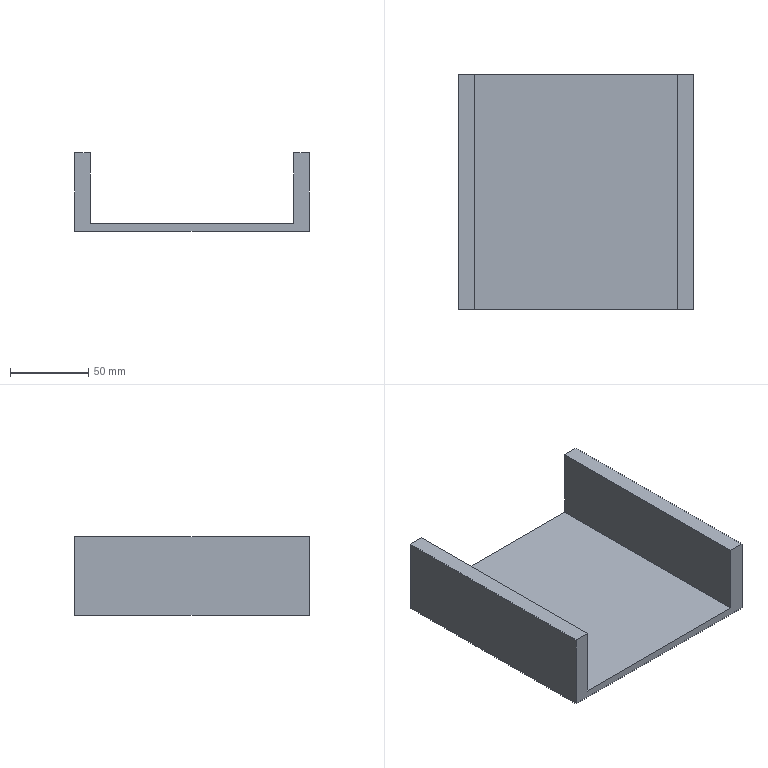Part | NX | features DATUM_CSYS 2, EXTRUDE 1, SKETCH 1 | 1 solid | 10 faces | box 150 x 150 x 50 mm | volume 247500 mm3 | plane 10
STEP:
#1=CARTESIAN_POINT('',(0.,0.,50.));
#2=VERTEX_POINT('',#1);
#3=CARTESIAN_POINT('',(10.,0.,50.));
#4=VERTEX_POINT('',#3);
#5=CARTESIAN_POINT('',(0.,0.,50.));
#6=DIRECTION('',(1.,0.,0.));
#7=VECTOR('',#6,1000.);
#8=LINE('',#5,#7);
#9=EDGE_CURVE('',#2,#4,#8,.T.);
#10=ORIENTED_EDGE('',*,*,#9,.T.);
#11=CARTESIAN_POINT('',(10.,150.,50.));
#12=VERTEX_POINT('',#11);
#13=CARTESIAN_POINT('',(10.,150.,50.));
#14=DIRECTION('',(0.,-1.,0.));
#15=VECTOR('',#14,1000.);
#16=LINE('',#13,#15);
#17=EDGE_CURVE('',#12,#4,#16,.T.);
#18=ORIENTED_EDGE('',*,*,#17,.F.);
#19=CARTESIAN_POINT('',(0.,150.,50.));
#20=VERTEX_POINT('',#19);
#21=CARTESIAN_POINT('',(0.,150.,50.));
#22=DIRECTION('',(1.,0.,0.));
#23=VECTOR('',#22,1000.);
#24=LINE('',#21,#23);
#25=EDGE_CURVE('',#20,#12,#24,.T.);
#26=ORIENTED_EDGE('',*,*,#25,.F.);
#27=CARTESIAN_POINT('',(0.,150.,50.));
#28=DIRECTION('',(0.,-1.,0.));
#29=VECTOR('',#28,1000.);
#30=LINE('',#27,#29);
#31=EDGE_CURVE('',#20,#2,#30,.T.);
#32=ORIENTED_EDGE('',*,*,#31,.T.);
#33=EDGE_LOOP('',(#10,#18,#26,#32));
#34=FACE_BOUND('',#33,.T.);
#35=CARTESIAN_POINT('',(0.,150.,50.));
#36=DIRECTION('',(0.,0.,-1.));
#37=DIRECTION('',(-1.,0.,0.));
#38=AXIS2_PLACEMENT_3D('',#35,#36,#37);
#39=PLANE('',#38);
#40=ADVANCED_FACE('',(#34),#39,.F.);
#41=CARTESIAN_POINT('',(10.,0.,5.));
#42=VERTEX_POINT('',#41);
#43=CARTESIAN_POINT('',(10.,0.,50.));
#44=DIRECTION('',(0.,0.,-1.));
#45=VECTOR('',#44,1000.);
#46=LINE('',#43,#45);
#47=EDGE_CURVE('',#4,#42,#46,.T.);
#48=ORIENTED_EDGE('',*,*,#47,.T.);
#49=CARTESIAN_POINT('',(10.,150.,5.));
#50=VERTEX_POINT('',#49);
#51=CARTESIAN_POINT('',(10.,150.,5.));
#52=DIRECTION('',(0.,-1.,0.));
#53=VECTOR('',#52,1000.);
#54=LINE('',#51,#53);
#55=EDGE_CURVE('',#50,#42,#54,.T.);
#56=ORIENTED_EDGE('',*,*,#55,.F.);
#57=CARTESIAN_POINT('',(10.,150.,50.));
#58=DIRECTION('',(0.,0.,-1.));
#59=VECTOR('',#58,1000.);
#60=LINE('',#57,#59);
#61=EDGE_CURVE('',#12,#50,#60,.T.);
#62=ORIENTED_EDGE('',*,*,#61,.F.);
#63=ORIENTED_EDGE('',*,*,#17,.T.);
#64=EDGE_LOOP('',(#48,#56,#62,#63));
#65=FACE_BOUND('',#64,.T.);
#66=CARTESIAN_POINT('',(10.,150.,50.));
#67=DIRECTION('',(-1.,0.,0.));
#68=DIRECTION('',(0.,0.,1.));
#69=AXIS2_PLACEMENT_3D('',#66,#67,#68);
#70=PLANE('',#69);
#71=ADVANCED_FACE('',(#65),#70,.F.);
#72=CARTESIAN_POINT('',(140.,0.,5.));
#73=VERTEX_POINT('',#72);
#74=CARTESIAN_POINT('',(10.,0.,5.));
#75=DIRECTION('',(1.,0.,0.));
#76=VECTOR('',#75,1000.);
#77=LINE('',#74,#76);
#78=EDGE_CURVE('',#42,#73,#77,.T.);
#79=ORIENTED_EDGE('',*,*,#78,.T.);
#80=CARTESIAN_POINT('',(140.,150.,5.));
#81=VERTEX_POINT('',#80);
#82=CARTESIAN_POINT('',(140.,150.,5.));
#83=DIRECTION('',(0.,-1.,0.));
#84=VECTOR('',#83,1000.);
#85=LINE('',#82,#84);
#86=EDGE_CURVE('',#81,#73,#85,.T.);
#87=ORIENTED_EDGE('',*,*,#86,.F.);
#88=CARTESIAN_POINT('',(10.,150.,5.));
#89=DIRECTION('',(1.,0.,0.));
#90=VECTOR('',#89,1000.);
#91=LINE('',#88,#90);
#92=EDGE_CURVE('',#50,#81,#91,.T.);
#93=ORIENTED_EDGE('',*,*,#92,.F.);
#94=ORIENTED_EDGE('',*,*,#55,.T.);
#95=EDGE_LOOP('',(#79,#87,#93,#94));
#96=FACE_BOUND('',#95,.T.);
#97=CARTESIAN_POINT('',(10.,150.,5.));
#98=DIRECTION('',(0.,0.,-1.));
#99=DIRECTION('',(-1.,0.,0.));
#100=AXIS2_PLACEMENT_3D('',#97,#98,#99);
#101=PLANE('',#100);
#102=ADVANCED_FACE('',(#96),#101,.F.);
#103=CARTESIAN_POINT('',(140.,0.,50.));
#104=VERTEX_POINT('',#103);
#105=CARTESIAN_POINT('',(140.,0.,5.));
#106=DIRECTION('',(0.,0.,1.));
#107=VECTOR('',#106,1000.);
#108=LINE('',#105,#107);
#109=EDGE_CURVE('',#73,#104,#108,.T.);
#110=ORIENTED_EDGE('',*,*,#109,.T.);
#111=CARTESIAN_POINT('',(140.,150.,50.));
#112=VERTEX_POINT('',#111);
#113=CARTESIAN_POINT('',(140.,150.,50.));
#114=DIRECTION('',(0.,-1.,0.));
#115=VECTOR('',#114,1000.);
#116=LINE('',#113,#115);
#117=EDGE_CURVE('',#112,#104,#116,.T.);
#118=ORIENTED_EDGE('',*,*,#117,.F.);
#119=CARTESIAN_POINT('',(140.,150.,5.));
#120=DIRECTION('',(0.,0.,1.));
#121=VECTOR('',#120,1000.);
#122=LINE('',#119,#121);
#123=EDGE_CURVE('',#81,#112,#122,.T.);
#124=ORIENTED_EDGE('',*,*,#123,.F.);
#125=ORIENTED_EDGE('',*,*,#86,.T.);
#126=EDGE_LOOP('',(#110,#118,#124,#125));
#127=FACE_BOUND('',#126,.T.);
#128=CARTESIAN_POINT('',(140.,150.,5.));
#129=DIRECTION('',(1.,0.,0.));
#130=DIRECTION('',(0.,0.,-1.));
#131=AXIS2_PLACEMENT_3D('',#128,#129,#130);
#132=PLANE('',#131);
#133=ADVANCED_FACE('',(#127),#132,.F.);
#134=CARTESIAN_POINT('',(150.,0.,50.));
#135=VERTEX_POINT('',#134);
#136=CARTESIAN_POINT('',(140.,0.,50.));
#137=DIRECTION('',(1.,0.,0.));
#138=VECTOR('',#137,1000.);
#139=LINE('',#136,#138);
#140=EDGE_CURVE('',#104,#135,#139,.T.);
#141=ORIENTED_EDGE('',*,*,#140,.T.);
#142=CARTESIAN_POINT('',(150.,150.,50.));
#143=VERTEX_POINT('',#142);
#144=CARTESIAN_POINT('',(150.,150.,50.));
#145=DIRECTION('',(0.,-1.,0.));
#146=VECTOR('',#145,1000.);
#147=LINE('',#144,#146);
#148=EDGE_CURVE('',#143,#135,#147,.T.);
#149=ORIENTED_EDGE('',*,*,#148,.F.);
#150=CARTESIAN_POINT('',(140.,150.,50.));
#151=DIRECTION('',(1.,0.,0.));
#152=VECTOR('',#151,1000.);
#153=LINE('',#150,#152);
#154=EDGE_CURVE('',#112,#143,#153,.T.);
#155=ORIENTED_EDGE('',*,*,#154,.F.);
#156=ORIENTED_EDGE('',*,*,#117,.T.);
#157=EDGE_LOOP('',(#141,#149,#155,#156));
#158=FACE_BOUND('',#157,.T.);
#159=CARTESIAN_POINT('',(140.,150.,50.));
#160=DIRECTION('',(0.,0.,-1.));
#161=DIRECTION('',(-1.,0.,0.));
#162=AXIS2_PLACEMENT_3D('',#159,#160,#161);
#163=PLANE('',#162);
#164=ADVANCED_FACE('',(#158),#163,.F.);
#165=CARTESIAN_POINT('',(150.,0.,0.));
#166=VERTEX_POINT('',#165);
#167=CARTESIAN_POINT('',(150.,0.,50.));
#168=DIRECTION('',(0.,0.,-1.));
#169=VECTOR('',#168,1000.);
#170=LINE('',#167,#169);
#171=EDGE_CURVE('',#135,#166,#170,.T.);
#172=ORIENTED_EDGE('',*,*,#171,.T.);
#173=CARTESIAN_POINT('',(150.,150.,0.));
#174=VERTEX_POINT('',#173);
#175=CARTESIAN_POINT('',(150.,150.,0.));
#176=DIRECTION('',(0.,-1.,0.));
#177=VECTOR('',#176,1000.);
#178=LINE('',#175,#177);
#179=EDGE_CURVE('',#174,#166,#178,.T.);
#180=ORIENTED_EDGE('',*,*,#179,.F.);
#181=CARTESIAN_POINT('',(150.,150.,50.));
#182=DIRECTION('',(0.,0.,-1.));
#183=VECTOR('',#182,1000.);
#184=LINE('',#181,#183);
#185=EDGE_CURVE('',#143,#174,#184,.T.);
#186=ORIENTED_EDGE('',*,*,#185,.F.);
#187=ORIENTED_EDGE('',*,*,#148,.T.);
#188=EDGE_LOOP('',(#172,#180,#186,#187));
#189=FACE_BOUND('',#188,.T.);
#190=CARTESIAN_POINT('',(150.,150.,50.));
#191=DIRECTION('',(-1.,0.,0.));
#192=DIRECTION('',(0.,0.,1.));
#193=AXIS2_PLACEMENT_3D('',#190,#191,#192);
#194=PLANE('',#193);
#195=ADVANCED_FACE('',(#189),#194,.F.);
#196=CARTESIAN_POINT('',(0.,0.,0.));
#197=VERTEX_POINT('',#196);
#198=CARTESIAN_POINT('',(150.,0.,0.));
#199=DIRECTION('',(-1.,0.,0.));
#200=VECTOR('',#199,1000.);
#201=LINE('',#198,#200);
#202=EDGE_CURVE('',#166,#197,#201,.T.);
#203=ORIENTED_EDGE('',*,*,#202,.T.);
#204=CARTESIAN_POINT('',(0.,150.,0.));
#205=VERTEX_POINT('',#204);
#206=CARTESIAN_POINT('',(0.,150.,0.));
#207=DIRECTION('',(0.,-1.,0.));
#208=VECTOR('',#207,1000.);
#209=LINE('',#206,#208);
#210=EDGE_CURVE('',#205,#197,#209,.T.);
#211=ORIENTED_EDGE('',*,*,#210,.F.);
#212=CARTESIAN_POINT('',(150.,150.,0.));
#213=DIRECTION('',(-1.,0.,0.));
#214=VECTOR('',#213,1000.);
#215=LINE('',#212,#214);
#216=EDGE_CURVE('',#174,#205,#215,.T.);
#217=ORIENTED_EDGE('',*,*,#216,.F.);
#218=ORIENTED_EDGE('',*,*,#179,.T.);
#219=EDGE_LOOP('',(#203,#211,#217,#218));
#220=FACE_BOUND('',#219,.T.);
#221=CARTESIAN_POINT('',(150.,150.,0.));
#222=DIRECTION('',(0.,0.,1.));
#223=DIRECTION('',(1.,0.,0.));
#224=AXIS2_PLACEMENT_3D('',#221,#222,#223);
#225=PLANE('',#224);
#226=ADVANCED_FACE('',(#220),#225,.F.);
#227=CARTESIAN_POINT('',(0.,0.,0.));
#228=DIRECTION('',(0.,0.,1.));
#229=VECTOR('',#228,1000.);
#230=LINE('',#227,#229);
#231=EDGE_CURVE('',#197,#2,#230,.T.);
#232=ORIENTED_EDGE('',*,*,#231,.T.);
#233=ORIENTED_EDGE('',*,*,#31,.F.);
#234=CARTESIAN_POINT('',(0.,150.,0.));
#235=DIRECTION('',(0.,0.,1.));
#236=VECTOR('',#235,1000.);
#237=LINE('',#234,#236);
#238=EDGE_CURVE('',#205,#20,#237,.T.);
#239=ORIENTED_EDGE('',*,*,#238,.F.);
#240=ORIENTED_EDGE('',*,*,#210,.T.);
#241=EDGE_LOOP('',(#232,#233,#239,#240));
#242=FACE_BOUND('',#241,.T.);
#243=CARTESIAN_POINT('',(0.,150.,0.));
#244=DIRECTION('',(1.,0.,0.));
#245=DIRECTION('',(0.,0.,-1.));
#246=AXIS2_PLACEMENT_3D('',#243,#244,#245);
#247=PLANE('',#246);
#248=ADVANCED_FACE('',(#242),#247,.F.);
#249=ORIENTED_EDGE('',*,*,#25,.T.);
#250=ORIENTED_EDGE('',*,*,#61,.T.);
#251=ORIENTED_EDGE('',*,*,#92,.T.);
#252=ORIENTED_EDGE('',*,*,#123,.T.);
#253=ORIENTED_EDGE('',*,*,#154,.T.);
#254=ORIENTED_EDGE('',*,*,#185,.T.);
#255=ORIENTED_EDGE('',*,*,#216,.T.);
#256=ORIENTED_EDGE('',*,*,#238,.T.);
#257=EDGE_LOOP('',(#249,#250,#251,#252,#253,#254,#255,#256));
#258=FACE_BOUND('',#257,.T.);
#259=CARTESIAN_POINT('',(0.,150.,0.));
#260=DIRECTION('',(0.,1.,0.));
#261=DIRECTION('',(0.,0.,1.));
#262=AXIS2_PLACEMENT_3D('',#259,#260,#261);
#263=PLANE('',#262);
#264=ADVANCED_FACE('',(#258),#263,.T.);
#265=ORIENTED_EDGE('',*,*,#9,.F.);
#266=ORIENTED_EDGE('',*,*,#231,.F.);
#267=ORIENTED_EDGE('',*,*,#202,.F.);
#268=ORIENTED_EDGE('',*,*,#171,.F.);
#269=ORIENTED_EDGE('',*,*,#140,.F.);
#270=ORIENTED_EDGE('',*,*,#109,.F.);
#271=ORIENTED_EDGE('',*,*,#78,.F.);
#272=ORIENTED_EDGE('',*,*,#47,.F.);
#273=EDGE_LOOP('',(#265,#266,#267,#268,#269,#270,#271,#272));
#274=FACE_BOUND('',#273,.T.);
#275=CARTESIAN_POINT('',(0.,0.,0.));
#276=DIRECTION('',(0.,1.,0.));
#277=DIRECTION('',(0.,0.,1.));
#278=AXIS2_PLACEMENT_3D('',#275,#276,#277);
#279=PLANE('',#278);
#280=ADVANCED_FACE('',(#274),#279,.F.);
#281=CLOSED_SHELL('',(#40,#71,#102,#133,#164,#195,#226,#248,#264,#280));
#282=MANIFOLD_SOLID_BREP('',#281);
#283=(LENGTH_UNIT()NAMED_UNIT(*)SI_UNIT(.MILLI.,.METRE.));
#284=UNCERTAINTY_MEASURE_WITH_UNIT(LENGTH_MEASURE(0.00001),#283,'','');
#285=(NAMED_UNIT(*)PLANE_ANGLE_UNIT()SI_UNIT($,.RADIAN.));
#286=(NAMED_UNIT(*)SI_UNIT($,.STERADIAN.)SOLID_ANGLE_UNIT());
#287=(GEOMETRIC_REPRESENTATION_CONTEXT(3)GLOBAL_UNCERTAINTY_ASSIGNED_CONTEXT((#284))GLOBAL_UNIT_ASSIGNED_CONTEXT((#283,#285,#286))REPRESENTATION_CONTEXT('',''));
#288=ADVANCED_BREP_SHAPE_REPRESENTATION('',(#282),#287);